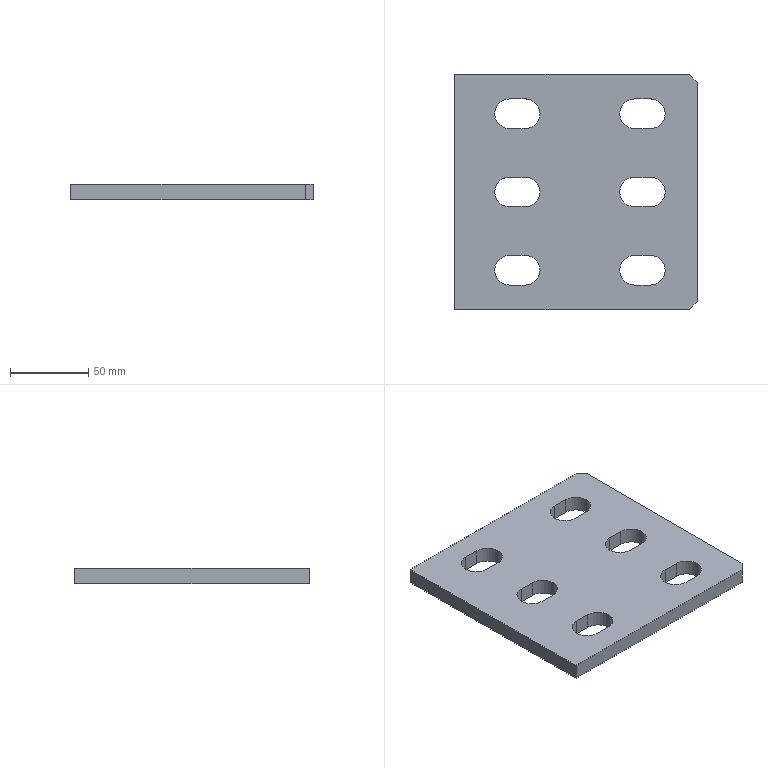Part | STEP file | 立柱翼Plate筋Plate-200 | 1 solid | 38 faces | box 155 x 150 x 10 mm | volume 203838 mm3 | plane 20 | cylinder 18 | commonest cylinder face diameters 19 x18